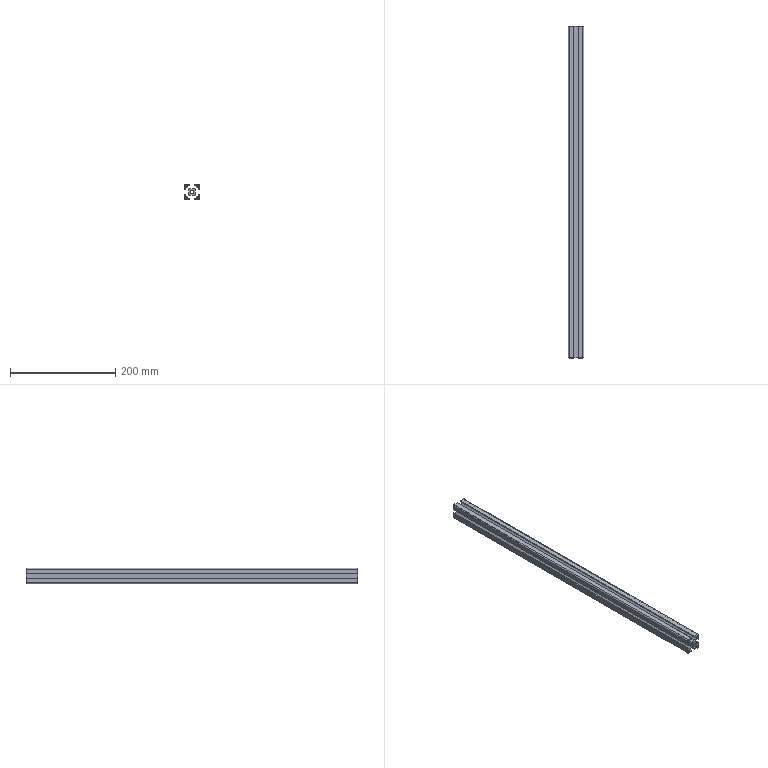Part | SolidWorks | features Extrusion 1 | 1 solid | 60 faces | box 30 x 630 x 30 mm | volume 209499 mm3 | plane 46 | cylinder 14 | commonest cylinder face diameters 4.2 x8 4 x4 6.8 x2